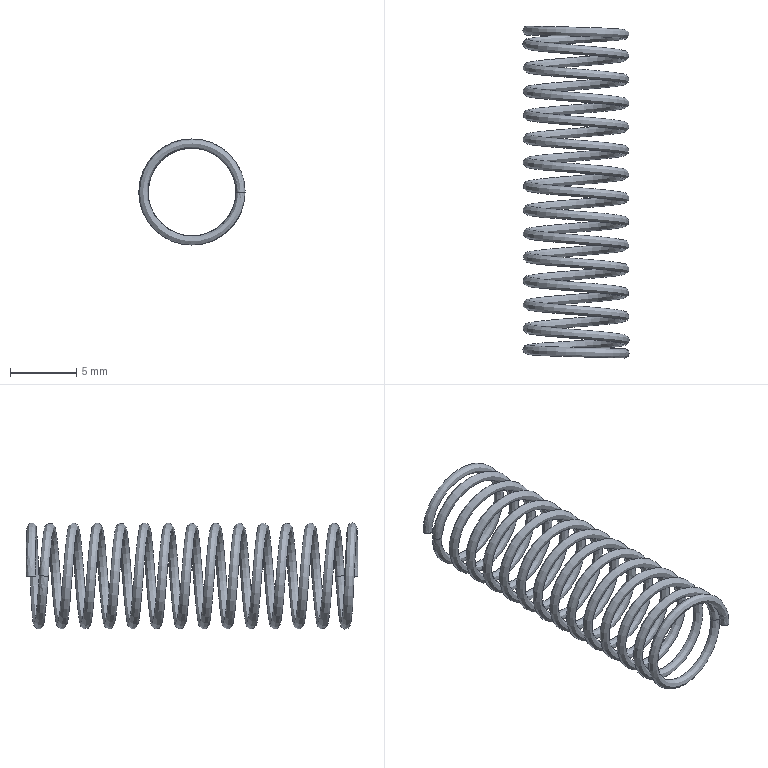Part | NX | features MI_WF_0301 2 | 1 solid | 5 faces | box 8 x 25 x 8 mm | volume 128.099 mm3 | spline 3 | plane 2